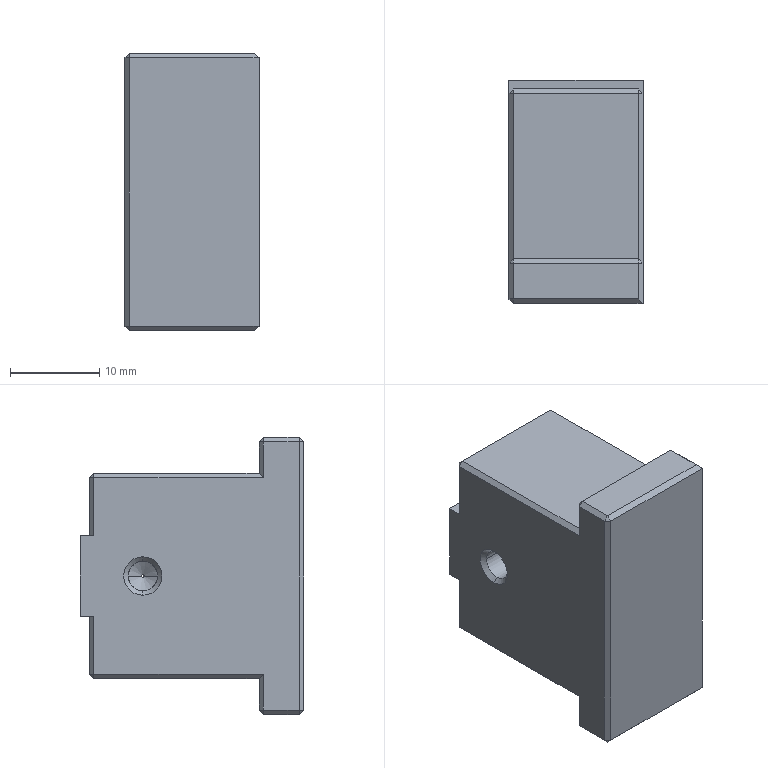Part | STEP file | 06-25 Cutter slider | 1 solid | 61 faces | box 15 x 25 x 31 mm | volume 8782 mm3 | plane 47 | cone 8 | cylinder 6 | commonest cylinder face diameters 2.5 x4 3.3 x2